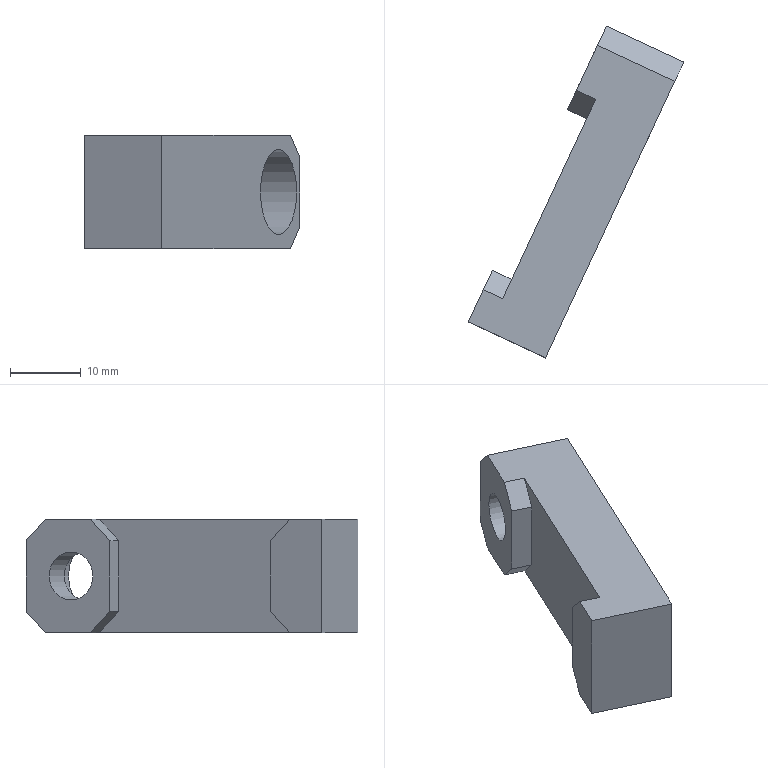Part | STEP file | gslz 2016.10.28-13_id454_x_t | 1 solid | 19 faces | box 30.316 x 46.762 x 16 mm | volume 6497 mm3 | plane 17 | cylinder 2 | commonest cylinder face diameters 6.8 x1 12 x1
STEP:
#1=CARTESIAN_POINT('',(0.,0.,0.));
#2=DIRECTION('',(0.,0.,1.));
#3=DIRECTION('',(1.,0.,0.));
#4=AXIS2_PLACEMENT_3D('',#1,#2,#3);
#5=CARTESIAN_POINT('',(887.546,-276.584,-28.));
#6=VERTEX_POINT('',#5);
#7=CARTESIAN_POINT('',(900.647,-248.489,-28.));
#8=VERTEX_POINT('',#7);
#9=CARTESIAN_POINT('',(891.35,-268.428,-28.));
#10=DIRECTION('',(0.4226,0.9063,0.));
#11=VECTOR('',#10,1.);
#12=LINE('',#9,#11);
#13=CARTESIAN_POINT('',(891.35,-268.428,-57.5));
#14=DIRECTION('',(0.9063,-0.4226,0.));
#15=DIRECTION('',(0.4226,0.9063,0.));
#16=AXIS2_PLACEMENT_3D('',#13,#14,#15);
#17=PLANE('',#16);
#18=CARTESIAN_POINT('',(0.,29.5));
#19=DIRECTION('',(1.,0.));
#20=VECTOR('',#19,1.);
#21=LINE('',#18,#20);
#22=(GEOMETRIC_REPRESENTATION_CONTEXT(2)PARAMETRIC_REPRESENTATION_CONTEXT()REPRESENTATION_CONTEXT('',''));
#23=DEFINITIONAL_REPRESENTATION('',(#21),#22);
#24=PCURVE('',#17,#23);
#25=CARTESIAN_POINT('',(900.413,-272.654,-28.));
#26=DIRECTION('',(0.,0.,-1.));
#27=DIRECTION('',(0.9397,-0.342,0.));
#28=AXIS2_PLACEMENT_3D('',#25,#26,#27);
#29=PLANE('',#28);
#30=CARTESIAN_POINT('',(-9.962,-0.8716));
#31=DIRECTION('',(0.08716,-0.9962));
#32=VECTOR('',#31,1.);
#33=LINE('',#30,#32);
#34=(GEOMETRIC_REPRESENTATION_CONTEXT(2)PARAMETRIC_REPRESENTATION_CONTEXT()REPRESENTATION_CONTEXT('',''));
#35=DEFINITIONAL_REPRESENTATION('',(#33),#34);
#36=PCURVE('',#29,#35);
#37=SURFACE_CURVE('',#12,(#24,#36),.PCURVE_S1.);
#38=EDGE_CURVE('',#6,#8,#37,.T.);
#39=ORIENTED_EDGE('',*,*,#38,.T.);
#40=CARTESIAN_POINT('',(899.379,-251.208,-31.));
#41=VERTEX_POINT('',#40);
#42=CARTESIAN_POINT('',(889.765,-271.826,-53.75));
#43=DIRECTION('',(0.2988,0.6409,0.7071));
#44=VECTOR('',#43,1.);
#45=LINE('',#42,#44);
#46=CARTESIAN_POINT('',(-3.75,3.75));
#47=DIRECTION('',(0.7071,0.7071));
#48=VECTOR('',#47,1.);
#49=LINE('',#46,#48);
#50=(GEOMETRIC_REPRESENTATION_CONTEXT(2)PARAMETRIC_REPRESENTATION_CONTEXT()REPRESENTATION_CONTEXT('',''));
#51=DEFINITIONAL_REPRESENTATION('',(#49),#50);
#52=PCURVE('',#17,#51);
#53=CARTESIAN_POINT('',(909.71,-252.715,-28.));
#54=DIRECTION('',(0.2988,0.6409,-0.7071));
#55=DIRECTION('',(-0.9063,0.4226,0.));
#56=AXIS2_PLACEMENT_3D('',#53,#54,#55);
#57=PLANE('',#56);
#58=CARTESIAN_POINT('',(10.,-36.416));
#59=DIRECTION('',(0.,1.));
#60=VECTOR('',#59,1.);
#61=LINE('',#58,#60);
#62=(GEOMETRIC_REPRESENTATION_CONTEXT(2)PARAMETRIC_REPRESENTATION_CONTEXT()REPRESENTATION_CONTEXT('',''));
#63=DEFINITIONAL_REPRESENTATION('',(#61),#62);
#64=PCURVE('',#57,#63);
#65=SURFACE_CURVE('',#45,(#52,#64),.PCURVE_S1.);
#66=EDGE_CURVE('',#41,#8,#65,.T.);
#67=ORIENTED_EDGE('',*,*,#66,.F.);
#68=CARTESIAN_POINT('',(899.379,-251.208,-41.));
#69=VERTEX_POINT('',#68);
#70=CARTESIAN_POINT('',(899.379,-251.208,-57.5));
#71=DIRECTION('',(0.,0.,1.));
#72=VECTOR('',#71,1.);
#73=LINE('',#70,#72);
#74=CARTESIAN_POINT('',(19.,0.));
#75=DIRECTION('',(0.,1.));
#76=VECTOR('',#75,1.);
#77=LINE('',#74,#76);
#78=(GEOMETRIC_REPRESENTATION_CONTEXT(2)PARAMETRIC_REPRESENTATION_CONTEXT()REPRESENTATION_CONTEXT('',''));
#79=DEFINITIONAL_REPRESENTATION('',(#77),#78);
#80=PCURVE('',#17,#79);
#81=CARTESIAN_POINT('',(907.536,-255.011,-36.));
#82=DIRECTION('',(0.4226,0.9063,0.));
#83=DIRECTION('',(0.9063,-0.4226,0.));
#84=AXIS2_PLACEMENT_3D('',#81,#82,#83);
#85=PLANE('',#84);
#86=CARTESIAN_POINT('',(-9.,21.5));
#87=DIRECTION('',(0.,-1.));
#88=VECTOR('',#87,1.);
#89=LINE('',#86,#88);
#90=(GEOMETRIC_REPRESENTATION_CONTEXT(2)PARAMETRIC_REPRESENTATION_CONTEXT()REPRESENTATION_CONTEXT('',''));
#91=DEFINITIONAL_REPRESENTATION('',(#89),#90);
#92=PCURVE('',#85,#91);
#93=SURFACE_CURVE('',#73,(#80,#92),.PCURVE_S1.);
#94=EDGE_CURVE('',#69,#41,#93,.T.);
#95=ORIENTED_EDGE('',*,*,#94,.F.);
#96=CARTESIAN_POINT('',(900.647,-248.489,-44.));
#97=VERTEX_POINT('',#96);
#98=CARTESIAN_POINT('',(898.851,-252.341,-39.75));
#99=DIRECTION('',(-0.2988,-0.6409,0.7071));
#100=VECTOR('',#99,1.);
#101=LINE('',#98,#100);
#102=CARTESIAN_POINT('',(17.75,17.75));
#103=DIRECTION('',(-0.7071,0.7071));
#104=VECTOR('',#103,1.);
#105=LINE('',#102,#104);
#106=(GEOMETRIC_REPRESENTATION_CONTEXT(2)PARAMETRIC_REPRESENTATION_CONTEXT()REPRESENTATION_CONTEXT('',''));
#107=DEFINITIONAL_REPRESENTATION('',(#105),#106);
#108=PCURVE('',#17,#107);
#109=CARTESIAN_POINT('',(907.536,-255.011,-41.));
#110=DIRECTION('',(-0.2988,-0.6409,-0.7071));
#111=DIRECTION('',(0.9063,-0.4226,0.));
#112=AXIS2_PLACEMENT_3D('',#109,#110,#111);
#113=PLANE('',#112);
#114=CARTESIAN_POINT('',(-9.,1.768));
#115=DIRECTION('',(0.,1.));
#116=VECTOR('',#115,1.);
#117=LINE('',#114,#116);
#118=(GEOMETRIC_REPRESENTATION_CONTEXT(2)PARAMETRIC_REPRESENTATION_CONTEXT()REPRESENTATION_CONTEXT('',''));
#119=DEFINITIONAL_REPRESENTATION('',(#117),#118);
#120=PCURVE('',#113,#119);
#121=SURFACE_CURVE('',#101,(#108,#120),.PCURVE_S1.);
#122=EDGE_CURVE('',#97,#69,#121,.T.);
#123=ORIENTED_EDGE('',*,*,#122,.F.);
#124=CARTESIAN_POINT('',(887.546,-276.584,-44.));
#125=VERTEX_POINT('',#124);
#126=CARTESIAN_POINT('',(891.35,-268.428,-44.));
#127=DIRECTION('',(0.4226,0.9063,0.));
#128=VECTOR('',#127,1.);
#129=LINE('',#126,#128);
#130=CARTESIAN_POINT('',(0.,13.5));
#131=DIRECTION('',(1.,0.));
#132=VECTOR('',#131,1.);
#133=LINE('',#130,#132);
#134=(GEOMETRIC_REPRESENTATION_CONTEXT(2)PARAMETRIC_REPRESENTATION_CONTEXT()REPRESENTATION_CONTEXT('',''));
#135=DEFINITIONAL_REPRESENTATION('',(#133),#134);
#136=PCURVE('',#17,#135);
#137=CARTESIAN_POINT('',(900.413,-272.654,-44.));
#138=DIRECTION('',(0.,0.,-1.));
#139=DIRECTION('',(0.9397,-0.342,0.));
#140=AXIS2_PLACEMENT_3D('',#137,#138,#139);
#141=PLANE('',#140);
#142=CARTESIAN_POINT('',(-9.962,-0.8716));
#143=DIRECTION('',(0.08716,-0.9962));
#144=VECTOR('',#143,1.);
#145=LINE('',#142,#144);
#146=(GEOMETRIC_REPRESENTATION_CONTEXT(2)PARAMETRIC_REPRESENTATION_CONTEXT()REPRESENTATION_CONTEXT('',''));
#147=DEFINITIONAL_REPRESENTATION('',(#145),#146);
#148=PCURVE('',#141,#147);
#149=SURFACE_CURVE('',#129,(#136,#148),.PCURVE_S1.);
#150=EDGE_CURVE('',#125,#97,#149,.T.);
#151=ORIENTED_EDGE('',*,*,#150,.F.);
#152=CARTESIAN_POINT('',(888.814,-273.865,-41.));
#153=VERTEX_POINT('',#152);
#154=CARTESIAN_POINT('',(886.595,-278.624,-46.25));
#155=DIRECTION('',(-0.2988,-0.6409,-0.7071));
#156=VECTOR('',#155,1.);
#157=LINE('',#154,#156);
#158=CARTESIAN_POINT('',(-11.25,11.25));
#159=DIRECTION('',(-0.7071,-0.7071));
#160=VECTOR('',#159,1.);
#161=LINE('',#158,#160);
#162=(GEOMETRIC_REPRESENTATION_CONTEXT(2)PARAMETRIC_REPRESENTATION_CONTEXT()REPRESENTATION_CONTEXT('',''));
#163=DEFINITIONAL_REPRESENTATION('',(#161),#162);
#164=PCURVE('',#17,#163);
#165=CARTESIAN_POINT('',(896.609,-280.811,-44.));
#166=DIRECTION('',(0.2988,0.6409,-0.7071));
#167=DIRECTION('',(0.9063,-0.4226,0.));
#168=AXIS2_PLACEMENT_3D('',#165,#166,#167);
#169=PLANE('',#168);
#170=CARTESIAN_POINT('',(-10.,3.182));
#171=DIRECTION('',(0.,1.));
#172=VECTOR('',#171,1.);
#173=LINE('',#170,#172);
#174=(GEOMETRIC_REPRESENTATION_CONTEXT(2)PARAMETRIC_REPRESENTATION_CONTEXT()REPRESENTATION_CONTEXT('',''));
#175=DEFINITIONAL_REPRESENTATION('',(#173),#174);
#176=PCURVE('',#169,#175);
#177=SURFACE_CURVE('',#157,(#164,#176),.PCURVE_S1.);
#178=EDGE_CURVE('',#153,#125,#177,.T.);
#179=ORIENTED_EDGE('',*,*,#178,.F.);
#180=CARTESIAN_POINT('',(888.814,-273.865,-31.));
#181=VERTEX_POINT('',#180);
#182=CARTESIAN_POINT('',(888.814,-273.865,-57.5));
#183=DIRECTION('',(0.,0.,1.));
#184=VECTOR('',#183,1.);
#185=LINE('',#182,#184);
#186=CARTESIAN_POINT('',(-6.,0.));
#187=DIRECTION('',(0.,1.));
#188=VECTOR('',#187,1.);
#189=LINE('',#186,#188);
#190=(GEOMETRIC_REPRESENTATION_CONTEXT(2)PARAMETRIC_REPRESENTATION_CONTEXT()REPRESENTATION_CONTEXT('',''));
#191=DEFINITIONAL_REPRESENTATION('',(#189),#190);
#192=PCURVE('',#17,#191);
#193=CARTESIAN_POINT('',(896.971,-277.669,-36.));
#194=DIRECTION('',(-0.4226,-0.9063,0.));
#195=DIRECTION('',(0.9063,-0.4226,0.));
#196=AXIS2_PLACEMENT_3D('',#193,#194,#195);
#197=PLANE('',#196);
#198=CARTESIAN_POINT('',(-9.,-21.5));
#199=DIRECTION('',(0.,1.));
#200=VECTOR('',#199,1.);
#201=LINE('',#198,#200);
#202=(GEOMETRIC_REPRESENTATION_CONTEXT(2)PARAMETRIC_REPRESENTATION_CONTEXT()REPRESENTATION_CONTEXT('',''));
#203=DEFINITIONAL_REPRESENTATION('',(#201),#202);
#204=PCURVE('',#197,#203);
#205=SURFACE_CURVE('',#185,(#192,#204),.PCURVE_S1.);
#206=EDGE_CURVE('',#153,#181,#205,.T.);
#207=ORIENTED_EDGE('',*,*,#206,.T.);
#208=CARTESIAN_POINT('',(895.681,-259.138,-47.25));
#209=DIRECTION('',(0.2988,0.6409,-0.7071));
#210=VECTOR('',#209,1.);
#211=LINE('',#208,#210);
#212=CARTESIAN_POINT('',(10.25,10.25));
#213=DIRECTION('',(0.7071,-0.7071));
#214=VECTOR('',#213,1.);
#215=LINE('',#212,#214);
#216=(GEOMETRIC_REPRESENTATION_CONTEXT(2)PARAMETRIC_REPRESENTATION_CONTEXT()REPRESENTATION_CONTEXT('',''));
#217=DEFINITIONAL_REPRESENTATION('',(#215),#216);
#218=PCURVE('',#17,#217);
#219=CARTESIAN_POINT('',(896.971,-277.669,-31.));
#220=DIRECTION('',(-0.2988,-0.6409,-0.7071));
#221=DIRECTION('',(-0.9063,0.4226,0.));
#222=AXIS2_PLACEMENT_3D('',#219,#220,#221);
#223=PLANE('',#222);
#224=CARTESIAN_POINT('',(9.,22.981));
#225=DIRECTION('',(0.,1.));
#226=VECTOR('',#225,1.);
#227=LINE('',#224,#226);
#228=(GEOMETRIC_REPRESENTATION_CONTEXT(2)PARAMETRIC_REPRESENTATION_CONTEXT()REPRESENTATION_CONTEXT('',''));
#229=DEFINITIONAL_REPRESENTATION('',(#227),#228);
#230=PCURVE('',#223,#229);
#231=SURFACE_CURVE('',#211,(#218,#230),.PCURVE_S1.);
#232=EDGE_CURVE('',#6,#181,#231,.T.);
#233=ORIENTED_EDGE('',*,*,#232,.F.);
#234=EDGE_LOOP('',(#39,#67,#95,#123,#151,#179,#207,#233));
#235=FACE_BOUND('',#234,.T.);
#236=ADVANCED_FACE('',(#235),#17,.F.);
#237=CARTESIAN_POINT('',(905.165,-243.534,-36.));
#238=VERTEX_POINT('',#237);
#239=CARTESIAN_POINT('',(903.728,-246.615,-36.));
#240=DIRECTION('',(0.9063,-0.4226,0.));
#241=DIRECTION('',(0.4226,0.9063,0.));
#242=AXIS2_PLACEMENT_3D('',#239,#240,#241);
#243=CIRCLE('',#242,3.4);
#244=CARTESIAN_POINT('',(817.628,-206.466,-36.));
#245=DIRECTION('',(-0.9063,0.4226,0.));
#246=DIRECTION('',(-0.4226,-0.9063,0.));
#247=AXIS2_PLACEMENT_3D('',#244,#245,#246);
#248=CYLINDRICAL_SURFACE('',#247,3.4);
#249=CARTESIAN_POINT('',(9.425,-95.));
#250=DIRECTION('',(-1.,0.));
#251=VECTOR('',#250,1.);
#252=LINE('',#249,#251);
#253=(GEOMETRIC_REPRESENTATION_CONTEXT(2)PARAMETRIC_REPRESENTATION_CONTEXT()REPRESENTATION_CONTEXT('',''));
#254=DEFINITIONAL_REPRESENTATION('',(#252),#253);
#255=PCURVE('',#248,#254);
#256=CARTESIAN_POINT('',(906.686,-240.271,-36.));
#257=DIRECTION('',(-0.9063,0.4226,0.));
#258=DIRECTION('',(-0.4226,-0.9063,0.));
#259=AXIS2_PLACEMENT_3D('',#256,#257,#258);
#260=PLANE('',#259);
#261=CARTESIAN_POINT('',(3.6,-0.000000001));
#262=CARTESIAN_POINT('',(3.6,5.889));
#263=CARTESIAN_POINT('',(8.7,2.944));
#264=CARTESIAN_POINT('',(13.8,0.000000001));
#265=CARTESIAN_POINT('',(8.7,-2.944));
#266=CARTESIAN_POINT('',(3.6,-5.889));
#267=CARTESIAN_POINT('',(3.6,-0.000000001));
#268=(BOUNDED_CURVE()B_SPLINE_CURVE(2,(#261,#262,#263,#264,#265,#266,#267),.UNSPECIFIED.,.T.,.F.)B_SPLINE_CURVE_WITH_KNOTS((1,2,2,2,2,1),(-2.094,0.,2.094,4.189,6.283,8.378),.UNSPECIFIED.)CURVE()GEOMETRIC_REPRESENTATION_ITEM()RATIONAL_B_SPLINE_CURVE((1.,0.5,1.,0.5,1.,0.5,1.))REPRESENTATION_ITEM(''));
#269=(GEOMETRIC_REPRESENTATION_CONTEXT(2)PARAMETRIC_REPRESENTATION_CONTEXT()REPRESENTATION_CONTEXT('',''));
#270=DEFINITIONAL_REPRESENTATION('',(#268),#269);
#271=PCURVE('',#260,#270);
#272=SURFACE_CURVE('',#243,(#255,#271),.PCURVE_S1.);
#273=EDGE_CURVE('',#238,#238,#272,.T.);
#274=ORIENTED_EDGE('',*,*,#273,.F.);
#275=CARTESIAN_POINT('',(900.633,-241.421,-36.));
#276=VERTEX_POINT('',#275);
#277=CARTESIAN_POINT('',(905.165,-243.534,-36.));
#278=CARTESIAN_POINT('',(900.633,-241.421,-36.));
#279=B_SPLINE_CURVE_WITH_KNOTS('',1,(#277,#278),.UNSPECIFIED.,.F.,.F.,(2,2),(-95.,-90.),.PIECEWISE_BEZIER_KNOTS.);
#280=CARTESIAN_POINT('',(9.425,0.));
#281=DIRECTION('',(0.,1.));
#282=VECTOR('',#281,1.);
#283=LINE('',#280,#282);
#284=(GEOMETRIC_REPRESENTATION_CONTEXT(2)PARAMETRIC_REPRESENTATION_CONTEXT()REPRESENTATION_CONTEXT('',''));
#285=DEFINITIONAL_REPRESENTATION('',(#283),#284);
#286=PCURVE('',#248,#285);
#287=CARTESIAN_POINT('',(3.142,0.));
#288=DIRECTION('',(0.,1.));
#289=VECTOR('',#288,1.);
#290=LINE('',#287,#289);
#291=(GEOMETRIC_REPRESENTATION_CONTEXT(2)PARAMETRIC_REPRESENTATION_CONTEXT()REPRESENTATION_CONTEXT('',''));
#292=DEFINITIONAL_REPRESENTATION('',(#290),#291);
#293=PCURVE('',#248,#292);
#294=SEAM_CURVE('',#279,(#286,#293),.PCURVE_S1.);
#295=EDGE_CURVE('',#238,#276,#294,.T.);
#296=ORIENTED_EDGE('',*,*,#295,.T.);
#297=CARTESIAN_POINT('',(899.196,-244.502,-36.));
#298=DIRECTION('',(-0.9063,0.4226,0.));
#299=DIRECTION('',(0.4226,0.9063,0.));
#300=AXIS2_PLACEMENT_3D('',#297,#298,#299);
#301=CIRCLE('',#300,3.4);
#302=CARTESIAN_POINT('',(3.142,-90.));
#303=DIRECTION('',(1.,0.));
#304=VECTOR('',#303,1.);
#305=LINE('',#302,#304);
#306=(GEOMETRIC_REPRESENTATION_CONTEXT(2)PARAMETRIC_REPRESENTATION_CONTEXT()REPRESENTATION_CONTEXT('',''));
#307=DEFINITIONAL_REPRESENTATION('',(#305),#306);
#308=PCURVE('',#248,#307);
#309=CARTESIAN_POINT('',(903.,-236.345,-57.5));
#310=DIRECTION('',(0.9063,-0.4226,0.));
#311=DIRECTION('',(-0.4226,-0.9063,0.));
#312=AXIS2_PLACEMENT_3D('',#309,#310,#311);
#313=PLANE('',#312);
#314=CARTESIAN_POINT('',(5.6,-21.5));
#315=CARTESIAN_POINT('',(5.6,-15.611));
#316=CARTESIAN_POINT('',(10.7,-18.556));
#317=CARTESIAN_POINT('',(15.8,-21.5));
#318=CARTESIAN_POINT('',(10.7,-24.444));
#319=CARTESIAN_POINT('',(5.6,-27.389));
#320=CARTESIAN_POINT('',(5.6,-21.5));
#321=(BOUNDED_CURVE()B_SPLINE_CURVE(2,(#314,#315,#316,#317,#318,#319,#320),.UNSPECIFIED.,.T.,.F.)B_SPLINE_CURVE_WITH_KNOTS((1,2,2,2,2,1),(-2.094,0.,2.094,4.189,6.283,8.378),.UNSPECIFIED.)CURVE()GEOMETRIC_REPRESENTATION_ITEM()RATIONAL_B_SPLINE_CURVE((1.,0.5,1.,0.5,1.,0.5,1.))REPRESENTATION_ITEM(''));
#322=(GEOMETRIC_REPRESENTATION_CONTEXT(2)PARAMETRIC_REPRESENTATION_CONTEXT()REPRESENTATION_CONTEXT('',''));
#323=DEFINITIONAL_REPRESENTATION('',(#321),#322);
#324=PCURVE('',#313,#323);
#325=SURFACE_CURVE('',#301,(#308,#324),.PCURVE_S1.);
#326=EDGE_CURVE('',#276,#276,#325,.T.);
#327=ORIENTED_EDGE('',*,*,#326,.F.);
#328=ORIENTED_EDGE('',*,*,#295,.F.);
#329=EDGE_LOOP('',(#274,#296,#327,#328));
#330=FACE_BOUND('',#329,.F.);
#331=ADVANCED_FACE('',(#330),#248,.F.);
#332=CARTESIAN_POINT('',(882.714,-279.848,-28.));
#333=VERTEX_POINT('',#332);
#334=CARTESIAN_POINT('',(884.827,-275.316,-28.));
#335=VERTEX_POINT('',#334);
#336=CARTESIAN_POINT('',(883.137,-278.942,-28.));
#337=DIRECTION('',(0.4226,0.9063,0.));
#338=VECTOR('',#337,1.);
#339=LINE('',#336,#338);
#340=CARTESIAN_POINT('',(-14.084,11.818));
#341=DIRECTION('',(0.08716,-0.9962));
#342=VECTOR('',#341,1.);
#343=LINE('',#340,#342);
#344=(GEOMETRIC_REPRESENTATION_CONTEXT(2)PARAMETRIC_REPRESENTATION_CONTEXT()REPRESENTATION_CONTEXT('',''));
#345=DEFINITIONAL_REPRESENTATION('',(#343),#344);
#346=PCURVE('',#29,#345);
#347=CARTESIAN_POINT('',(885.25,-274.41,-57.5));
#348=DIRECTION('',(0.9063,-0.4226,0.));
#349=DIRECTION('',(0.4226,0.9063,0.));
#350=AXIS2_PLACEMENT_3D('',#347,#348,#349);
#351=PLANE('',#350);
#352=CARTESIAN_POINT('',(-5.,29.5));
#353=DIRECTION('',(1.,0.));
#354=VECTOR('',#353,1.);
#355=LINE('',#352,#354);
#356=(GEOMETRIC_REPRESENTATION_CONTEXT(2)PARAMETRIC_REPRESENTATION_CONTEXT()REPRESENTATION_CONTEXT('',''));
#357=DEFINITIONAL_REPRESENTATION('',(#355),#356);
#358=PCURVE('',#351,#357);
#359=SURFACE_CURVE('',#339,(#346,#358),.PCURVE_S1.);
#360=EDGE_CURVE('',#333,#335,#359,.T.);
#361=ORIENTED_EDGE('',*,*,#360,.F.);
#362=CARTESIAN_POINT('',(893.59,-284.919,-28.));
#363=VERTEX_POINT('',#362);
#364=CARTESIAN_POINT('',(894.496,-285.342,-28.));
#365=DIRECTION('',(0.9063,-0.4226,0.));
#366=VECTOR('',#365,1.);
#367=LINE('',#364,#366);
#368=CARTESIAN_POINT('',(-1.22,13.947));
#369=DIRECTION('',(0.9962,0.08716));
#370=VECTOR('',#369,1.);
#371=LINE('',#368,#370);
#372=(GEOMETRIC_REPRESENTATION_CONTEXT(2)PARAMETRIC_REPRESENTATION_CONTEXT()REPRESENTATION_CONTEXT('',''));
#373=DEFINITIONAL_REPRESENTATION('',(#371),#372);
#374=PCURVE('',#29,#373);
#375=CARTESIAN_POINT('',(894.496,-285.342,-57.5));
#376=DIRECTION('',(-0.4226,-0.9063,0.));
#377=DIRECTION('',(0.9063,-0.4226,0.));
#378=AXIS2_PLACEMENT_3D('',#375,#376,#377);
#379=PLANE('',#378);
#380=CARTESIAN_POINT('',(0.,29.5));
#381=DIRECTION('',(1.,0.));
#382=VECTOR('',#381,1.);
#383=LINE('',#380,#382);
#384=(GEOMETRIC_REPRESENTATION_CONTEXT(2)PARAMETRIC_REPRESENTATION_CONTEXT()REPRESENTATION_CONTEXT('',''));
#385=DEFINITIONAL_REPRESENTATION('',(#383),#384);
#386=PCURVE('',#379,#385);
#387=SURFACE_CURVE('',#367,(#374,#386),.PCURVE_S1.);
#388=EDGE_CURVE('',#333,#363,#387,.T.);
#389=ORIENTED_EDGE('',*,*,#388,.T.);
#390=CARTESIAN_POINT('',(911.762,-245.948,-28.));
#391=VERTEX_POINT('',#390);
#392=CARTESIAN_POINT('',(899.506,-272.231,-28.));
#393=DIRECTION('',(0.4226,0.9063,0.));
#394=VECTOR('',#393,1.);
#395=LINE('',#392,#394);
#396=CARTESIAN_POINT('',(-0.9962,-0.08716));
#397=DIRECTION('',(0.08716,-0.9962));
#398=VECTOR('',#397,1.);
#399=LINE('',#396,#398);
#400=(GEOMETRIC_REPRESENTATION_CONTEXT(2)PARAMETRIC_REPRESENTATION_CONTEXT()REPRESENTATION_CONTEXT('',''));
#401=DEFINITIONAL_REPRESENTATION('',(#399),#400);
#402=PCURVE('',#29,#401);
#403=CARTESIAN_POINT('',(899.506,-272.231,-57.5));
#404=DIRECTION('',(0.9063,-0.4226,0.));
#405=DIRECTION('',(0.4226,0.9063,0.));
#406=AXIS2_PLACEMENT_3D('',#403,#404,#405);
#407=PLANE('',#406);
#408=CARTESIAN_POINT('',(0.,29.5));
#409=DIRECTION('',(1.,0.));
#410=VECTOR('',#409,1.);
#411=LINE('',#408,#410);
#412=(GEOMETRIC_REPRESENTATION_CONTEXT(2)PARAMETRIC_REPRESENTATION_CONTEXT()REPRESENTATION_CONTEXT('',''));
#413=DEFINITIONAL_REPRESENTATION('',(#411),#412);
#414=PCURVE('',#407,#413);
#415=SURFACE_CURVE('',#395,(#402,#414),.PCURVE_S1.);
#416=EDGE_CURVE('',#363,#391,#415,.T.);
#417=ORIENTED_EDGE('',*,*,#416,.T.);
#418=CARTESIAN_POINT('',(900.887,-240.877,-28.));
#419=VERTEX_POINT('',#418);
#420=CARTESIAN_POINT('',(900.887,-240.877,-28.));
#421=DIRECTION('',(-0.9063,0.4226,0.));
#422=VECTOR('',#421,1.);
#423=LINE('',#420,#422);
#424=CARTESIAN_POINT('',(-10.423,-30.023));
#425=DIRECTION('',(-0.9962,-0.08716));
#426=VECTOR('',#425,1.);
#427=LINE('',#424,#426);
#428=(GEOMETRIC_REPRESENTATION_CONTEXT(2)PARAMETRIC_REPRESENTATION_CONTEXT()REPRESENTATION_CONTEXT('',''));
#429=DEFINITIONAL_REPRESENTATION('',(#427),#428);
#430=PCURVE('',#29,#429);
#431=CARTESIAN_POINT('',(913.936,-243.652,-31.));
#432=DIRECTION('',(0.2988,0.6409,0.7071));
#433=DIRECTION('',(-0.9063,0.4226,0.));
#434=AXIS2_PLACEMENT_3D('',#431,#432,#433);
#435=PLANE('',#434);
#436=CARTESIAN_POINT('',(13.,4.243));
#437=DIRECTION('',(1.,0.));
#438=VECTOR('',#437,1.);
#439=LINE('',#436,#438);
#440=(GEOMETRIC_REPRESENTATION_CONTEXT(2)PARAMETRIC_REPRESENTATION_CONTEXT()REPRESENTATION_CONTEXT('',''));
#441=DEFINITIONAL_REPRESENTATION('',(#439),#440);
#442=PCURVE('',#435,#441);
#443=SURFACE_CURVE('',#423,(#430,#442),.PCURVE_S1.);
#444=EDGE_CURVE('',#391,#419,#443,.T.);
#445=ORIENTED_EDGE('',*,*,#444,.T.);
#446=CARTESIAN_POINT('',(897.928,-247.221,-28.));
#447=VERTEX_POINT('',#446);
#448=CARTESIAN_POINT('',(905.113,-231.814,-28.));
#449=DIRECTION('',(-0.4226,-0.9063,0.));
#450=VECTOR('',#449,1.);
#451=LINE('',#448,#450);
#452=CARTESIAN_POINT('',(-9.551,-39.985));
#453=DIRECTION('',(-0.08716,0.9962));
#454=VECTOR('',#453,1.);
#455=LINE('',#452,#454);
#456=(GEOMETRIC_REPRESENTATION_CONTEXT(2)PARAMETRIC_REPRESENTATION_CONTEXT()REPRESENTATION_CONTEXT('',''));
#457=DEFINITIONAL_REPRESENTATION('',(#455),#456);
#458=PCURVE('',#29,#457);
#459=CARTESIAN_POINT('',(-5.,-29.5));
#460=DIRECTION('',(1.,0.));
#461=VECTOR('',#460,1.);
#462=LINE('',#459,#461);
#463=(GEOMETRIC_REPRESENTATION_CONTEXT(2)PARAMETRIC_REPRESENTATION_CONTEXT()REPRESENTATION_CONTEXT('',''));
#464=DEFINITIONAL_REPRESENTATION('',(#462),#463);
#465=PCURVE('',#313,#464);
#466=SURFACE_CURVE('',#451,(#458,#465),.PCURVE_S1.);
#467=EDGE_CURVE('',#419,#447,#466,.T.);
#468=ORIENTED_EDGE('',*,*,#467,.T.);
#469=CARTESIAN_POINT('',(909.71,-252.715,-28.));
#470=DIRECTION('',(-0.9063,0.4226,0.));
#471=VECTOR('',#470,1.);
#472=LINE('',#469,#471);
#473=CARTESIAN_POINT('',(1.917,-21.916));
#474=DIRECTION('',(-0.9962,-0.08716));
#475=VECTOR('',#474,1.);
#476=LINE('',#473,#475);
#477=(GEOMETRIC_REPRESENTATION_CONTEXT(2)PARAMETRIC_REPRESENTATION_CONTEXT()REPRESENTATION_CONTEXT('',''));
#478=DEFINITIONAL_REPRESENTATION('',(#476),#477);
#479=PCURVE('',#29,#478);
#480=CARTESIAN_POINT('',(0.,0.));
#481=DIRECTION('',(1.,0.));
#482=VECTOR('',#481,1.);
#483=LINE('',#480,#482);
#484=(GEOMETRIC_REPRESENTATION_CONTEXT(2)PARAMETRIC_REPRESENTATION_CONTEXT()REPRESENTATION_CONTEXT('',''));
#485=DEFINITIONAL_REPRESENTATION('',(#483),#484);
#486=PCURVE('',#57,#485);
#487=SURFACE_CURVE('',#472,(#479,#486),.PCURVE_S1.);
#488=EDGE_CURVE('',#8,#447,#487,.T.);
#489=ORIENTED_EDGE('',*,*,#488,.F.);
#490=ORIENTED_EDGE('',*,*,#38,.F.);
#491=CARTESIAN_POINT('',(896.609,-280.811,-28.));
#492=DIRECTION('',(0.9063,-0.4226,0.));
#493=VECTOR('',#492,1.);
#494=LINE('',#491,#493);
#495=CARTESIAN_POINT('',(-0.7844,8.966));
#496=DIRECTION('',(0.9962,0.08716));
#497=VECTOR('',#496,1.);
#498=LINE('',#495,#497);
#499=(GEOMETRIC_REPRESENTATION_CONTEXT(2)PARAMETRIC_REPRESENTATION_CONTEXT()REPRESENTATION_CONTEXT('',''));
#500=DEFINITIONAL_REPRESENTATION('',(#498),#499);
#501=PCURVE('',#29,#500);
#502=CARTESIAN_POINT('',(-1.,-4.243));
#503=DIRECTION('',(-1.,0.));
#504=VECTOR('',#503,1.);
#505=LINE('',#502,#504);
#506=(GEOMETRIC_REPRESENTATION_CONTEXT(2)PARAMETRIC_REPRESENTATION_CONTEXT()REPRESENTATION_CONTEXT('',''));
#507=DEFINITIONAL_REPRESENTATION('',(#505),#506);
#508=PCURVE('',#223,#507);
#509=SURFACE_CURVE('',#494,(#501,#508),.PCURVE_S1.);
#510=EDGE_CURVE('',#335,#6,#509,.T.);
#511=ORIENTED_EDGE('',*,*,#510,.F.);
#512=EDGE_LOOP('',(#361,#389,#417,#445,#468,#489,#490,#511));
#513=FACE_BOUND('',#512,.T.);
#514=ADVANCED_FACE('',(#513),#29,.F.);
#515=CARTESIAN_POINT('',(882.714,-279.848,-44.));
#516=VERTEX_POINT('',#515);
#517=CARTESIAN_POINT('',(882.714,-279.848,-57.5));
#518=DIRECTION('',(0.,0.,-1.));
#519=VECTOR('',#518,1.);
#520=LINE('',#517,#519);
#521=CARTESIAN_POINT('',(-13.,0.));
#522=DIRECTION('',(0.,-1.));
#523=VECTOR('',#522,1.);
#524=LINE('',#521,#523);
#525=(GEOMETRIC_REPRESENTATION_CONTEXT(2)PARAMETRIC_REPRESENTATION_CONTEXT()REPRESENTATION_CONTEXT('',''));
#526=DEFINITIONAL_REPRESENTATION('',(#524),#525);
#527=PCURVE('',#379,#526);
#528=CARTESIAN_POINT('',(-6.,0.));
#529=DIRECTION('',(0.,-1.));
#530=VECTOR('',#529,1.);
#531=LINE('',#528,#530);
#532=(GEOMETRIC_REPRESENTATION_CONTEXT(2)PARAMETRIC_REPRESENTATION_CONTEXT()REPRESENTATION_CONTEXT('',''));
#533=DEFINITIONAL_REPRESENTATION('',(#531),#532);
#534=PCURVE('',#351,#533);
#535=SURFACE_CURVE('',#520,(#527,#534),.PCURVE_S1.);
#536=EDGE_CURVE('',#333,#516,#535,.T.);
#537=ORIENTED_EDGE('',*,*,#536,.T.);
#538=CARTESIAN_POINT('',(893.59,-284.919,-44.));
#539=VERTEX_POINT('',#538);
#540=CARTESIAN_POINT('',(894.496,-285.342,-44.));
#541=DIRECTION('',(0.9063,-0.4226,0.));
#542=VECTOR('',#541,1.);
#543=LINE('',#540,#542);
#544=CARTESIAN_POINT('',(0.,13.5));
#545=DIRECTION('',(1.,0.));
#546=VECTOR('',#545,1.);
#547=LINE('',#544,#546);
#548=(GEOMETRIC_REPRESENTATION_CONTEXT(2)PARAMETRIC_REPRESENTATION_CONTEXT()REPRESENTATION_CONTEXT('',''));
#549=DEFINITIONAL_REPRESENTATION('',(#547),#548);
#550=PCURVE('',#379,#549);
#551=CARTESIAN_POINT('',(-1.22,13.947));
#552=DIRECTION('',(0.9962,0.08716));
#553=VECTOR('',#552,1.);
#554=LINE('',#551,#553);
#555=(GEOMETRIC_REPRESENTATION_CONTEXT(2)PARAMETRIC_REPRESENTATION_CONTEXT()REPRESENTATION_CONTEXT('',''));
#556=DEFINITIONAL_REPRESENTATION('',(#554),#555);
#557=PCURVE('',#141,#556);
#558=SURFACE_CURVE('',#543,(#550,#557),.PCURVE_S1.);
#559=EDGE_CURVE('',#516,#539,#558,.T.);
#560=ORIENTED_EDGE('',*,*,#559,.T.);
#561=CARTESIAN_POINT('',(893.59,-284.919,-57.5));
#562=DIRECTION('',(0.,0.,1.));
#563=VECTOR('',#562,1.);
#564=LINE('',#561,#563);
#565=CARTESIAN_POINT('',(-1.,0.));
#566=DIRECTION('',(0.,1.));
#567=VECTOR('',#566,1.);
#568=LINE('',#565,#567);
#569=(GEOMETRIC_REPRESENTATION_CONTEXT(2)PARAMETRIC_REPRESENTATION_CONTEXT()REPRESENTATION_CONTEXT('',''));
#570=DEFINITIONAL_REPRESENTATION('',(#568),#569);
#571=PCURVE('',#379,#570);
#572=CARTESIAN_POINT('',(-14.,0.));
#573=DIRECTION('',(0.,1.));
#574=VECTOR('',#573,1.);
#575=LINE('',#572,#574);
#576=(GEOMETRIC_REPRESENTATION_CONTEXT(2)PARAMETRIC_REPRESENTATION_CONTEXT()REPRESENTATION_CONTEXT('',''));
#577=DEFINITIONAL_REPRESENTATION('',(#575),#576);
#578=PCURVE('',#407,#577);
#579=SURFACE_CURVE('',#564,(#571,#578),.PCURVE_S1.);
#580=EDGE_CURVE('',#539,#363,#579,.T.);
#581=ORIENTED_EDGE('',*,*,#580,.T.);
#582=ORIENTED_EDGE('',*,*,#388,.F.);
#583=EDGE_LOOP('',(#537,#560,#581,#582));
#584=FACE_BOUND('',#583,.T.);
#585=ADVANCED_FACE('',(#584),#379,.T.);
#586=ORIENTED_EDGE('',*,*,#150,.T.);
#587=CARTESIAN_POINT('',(897.928,-247.221,-44.));
#588=VERTEX_POINT('',#587);
#589=CARTESIAN_POINT('',(900.647,-248.489,-44.));
#590=DIRECTION('',(0.9063,-0.4226,0.));
#591=VECTOR('',#590,1.);
#592=LINE('',#589,#591);
#593=CARTESIAN_POINT('',(-8.045,-22.788));
#594=DIRECTION('',(0.9962,0.08716));
#595=VECTOR('',#594,1.);
#596=LINE('',#593,#595);
#597=(GEOMETRIC_REPRESENTATION_CONTEXT(2)PARAMETRIC_REPRESENTATION_CONTEXT()REPRESENTATION_CONTEXT('',''));
#598=DEFINITIONAL_REPRESENTATION('',(#596),#597);
#599=PCURVE('',#141,#598);
#600=CARTESIAN_POINT('',(-9.,-4.243));
#601=DIRECTION('',(1.,0.));
#602=VECTOR('',#601,1.);
#603=LINE('',#600,#602);
#604=(GEOMETRIC_REPRESENTATION_CONTEXT(2)PARAMETRIC_REPRESENTATION_CONTEXT()REPRESENTATION_CONTEXT('',''));
#605=DEFINITIONAL_REPRESENTATION('',(#603),#604);
#606=PCURVE('',#113,#605);
#607=SURFACE_CURVE('',#592,(#599,#606),.PCURVE_S1.);
#608=EDGE_CURVE('',#588,#97,#607,.T.);
#609=ORIENTED_EDGE('',*,*,#608,.F.);
#610=CARTESIAN_POINT('',(900.887,-240.877,-44.));
#611=VERTEX_POINT('',#610);
#612=CARTESIAN_POINT('',(905.113,-231.814,-44.));
#613=DIRECTION('',(-0.4226,-0.9063,0.));
#614=VECTOR('',#613,1.);
#615=LINE('',#612,#614);
#616=CARTESIAN_POINT('',(-9.551,-39.985));
#617=DIRECTION('',(-0.08716,0.9962));
#618=VECTOR('',#617,1.);
#619=LINE('',#616,#618);
#620=(GEOMETRIC_REPRESENTATION_CONTEXT(2)PARAMETRIC_REPRESENTATION_CONTEXT()REPRESENTATION_CONTEXT('',''));
#621=DEFINITIONAL_REPRESENTATION('',(#619),#620);
#622=PCURVE('',#141,#621);
#623=CARTESIAN_POINT('',(-5.,-13.5));
#624=DIRECTION('',(1.,0.));
#625=VECTOR('',#624,1.);
#626=LINE('',#623,#625);
#627=(GEOMETRIC_REPRESENTATION_CONTEXT(2)PARAMETRIC_REPRESENTATION_CONTEXT()REPRESENTATION_CONTEXT('',''));
#628=DEFINITIONAL_REPRESENTATION('',(#626),#627);
#629=PCURVE('',#313,#628);
#630=SURFACE_CURVE('',#615,(#622,#629),.PCURVE_S1.);
#631=EDGE_CURVE('',#611,#588,#630,.T.);
#632=ORIENTED_EDGE('',*,*,#631,.F.);
#633=CARTESIAN_POINT('',(911.762,-245.948,-44.));
#634=VERTEX_POINT('',#633);
#635=CARTESIAN_POINT('',(912.669,-246.371,-44.));
#636=DIRECTION('',(0.9063,-0.4226,0.));
#637=VECTOR('',#636,1.);
#638=LINE('',#635,#637);
#639=CARTESIAN_POINT('',(2.528,-28.89));
#640=DIRECTION('',(0.9962,0.08716));
#641=VECTOR('',#640,1.);
#642=LINE('',#639,#641);
#643=(GEOMETRIC_REPRESENTATION_CONTEXT(2)PARAMETRIC_REPRESENTATION_CONTEXT()REPRESENTATION_CONTEXT('',''));
#644=DEFINITIONAL_REPRESENTATION('',(#642),#643);
#645=PCURVE('',#141,#644);
#646=CARTESIAN_POINT('',(912.669,-246.371,-44.));
#647=DIRECTION('',(-0.2988,-0.6409,0.7071));
#648=DIRECTION('',(0.9063,-0.4226,0.));
#649=AXIS2_PLACEMENT_3D('',#646,#647,#648);
#650=PLANE('',#649);
#651=CARTESIAN_POINT('',(0.,0.));
#652=DIRECTION('',(1.,0.));
#653=VECTOR('',#652,1.);
#654=LINE('',#651,#653);
#655=(GEOMETRIC_REPRESENTATION_CONTEXT(2)PARAMETRIC_REPRESENTATION_CONTEXT()REPRESENTATION_CONTEXT('',''));
#656=DEFINITIONAL_REPRESENTATION('',(#654),#655);
#657=PCURVE('',#650,#656);
#658=SURFACE_CURVE('',#638,(#645,#657),.PCURVE_S1.);
#659=EDGE_CURVE('',#611,#634,#658,.T.);
#660=ORIENTED_EDGE('',*,*,#659,.T.);
#661=CARTESIAN_POINT('',(899.506,-272.231,-44.));
#662=DIRECTION('',(0.4226,0.9063,0.));
#663=VECTOR('',#662,1.);
#664=LINE('',#661,#663);
#665=CARTESIAN_POINT('',(-0.9962,-0.08716));
#666=DIRECTION('',(0.08716,-0.9962));
#667=VECTOR('',#666,1.);
#668=LINE('',#665,#667);
#669=(GEOMETRIC_REPRESENTATION_CONTEXT(2)PARAMETRIC_REPRESENTATION_CONTEXT()REPRESENTATION_CONTEXT('',''));
#670=DEFINITIONAL_REPRESENTATION('',(#668),#669);
#671=PCURVE('',#141,#670);
#672=CARTESIAN_POINT('',(0.,13.5));
#673=DIRECTION('',(1.,0.));
#674=VECTOR('',#673,1.);
#675=LINE('',#672,#674);
#676=(GEOMETRIC_REPRESENTATION_CONTEXT(2)PARAMETRIC_REPRESENTATION_CONTEXT()REPRESENTATION_CONTEXT('',''));
#677=DEFINITIONAL_REPRESENTATION('',(#675),#676);
#678=PCURVE('',#407,#677);
#679=SURFACE_CURVE('',#664,(#671,#678),.PCURVE_S1.);
#680=EDGE_CURVE('',#539,#634,#679,.T.);
#681=ORIENTED_EDGE('',*,*,#680,.F.);
#682=ORIENTED_EDGE('',*,*,#559,.F.);
#683=CARTESIAN_POINT('',(884.827,-275.316,-44.));
#684=VERTEX_POINT('',#683);
#685=CARTESIAN_POINT('',(883.137,-278.942,-44.));
#686=DIRECTION('',(0.4226,0.9063,0.));
#687=VECTOR('',#686,1.);
#688=LINE('',#685,#687);
#689=CARTESIAN_POINT('',(-14.084,11.818));
#690=DIRECTION('',(0.08716,-0.9962));
#691=VECTOR('',#690,1.);
#692=LINE('',#689,#691);
#693=(GEOMETRIC_REPRESENTATION_CONTEXT(2)PARAMETRIC_REPRESENTATION_CONTEXT()REPRESENTATION_CONTEXT('',''));
#694=DEFINITIONAL_REPRESENTATION('',(#692),#693);
#695=PCURVE('',#141,#694);
#696=CARTESIAN_POINT('',(-5.,13.5));
#697=DIRECTION('',(1.,0.));
#698=VECTOR('',#697,1.);
#699=LINE('',#696,#698);
#700=(GEOMETRIC_REPRESENTATION_CONTEXT(2)PARAMETRIC_REPRESENTATION_CONTEXT()REPRESENTATION_CONTEXT('',''));
#701=DEFINITIONAL_REPRESENTATION('',(#699),#700);
#702=PCURVE('',#351,#701);
#703=SURFACE_CURVE('',#688,(#695,#702),.PCURVE_S1.);
#704=EDGE_CURVE('',#516,#684,#703,.T.);
#705=ORIENTED_EDGE('',*,*,#704,.T.);
#706=CARTESIAN_POINT('',(884.827,-275.316,-44.));
#707=DIRECTION('',(-0.9063,0.4226,0.));
#708=VECTOR('',#707,1.);
#709=LINE('',#706,#708);
#710=CARTESIAN_POINT('',(-13.735,7.833));
#711=DIRECTION('',(-0.9962,-0.08716));
#712=VECTOR('',#711,1.);
#713=LINE('',#710,#712);
#714=(GEOMETRIC_REPRESENTATION_CONTEXT(2)PARAMETRIC_REPRESENTATION_CONTEXT()REPRESENTATION_CONTEXT('',''));
#715=DEFINITIONAL_REPRESENTATION('',(#713),#714);
#716=PCURVE('',#141,#715);
#717=CARTESIAN_POINT('',(-13.,0.));
#718=DIRECTION('',(-1.,0.));
#719=VECTOR('',#718,1.);
#720=LINE('',#717,#719);
#721=(GEOMETRIC_REPRESENTATION_CONTEXT(2)PARAMETRIC_REPRESENTATION_CONTEXT()REPRESENTATION_CONTEXT('',''));
#722=DEFINITIONAL_REPRESENTATION('',(#720),#721);
#723=PCURVE('',#169,#722);
#724=SURFACE_CURVE('',#709,(#716,#723),.PCURVE_S1.);
#725=EDGE_CURVE('',#125,#684,#724,.T.);
#726=ORIENTED_EDGE('',*,*,#725,.F.);
#727=EDGE_LOOP('',(#586,#609,#632,#660,#681,#682,#705,#726));
#728=FACE_BOUND('',#727,.T.);
#729=ADVANCED_FACE('',(#728),#141,.T.);
#730=ORIENTED_EDGE('',*,*,#580,.F.);
#731=ORIENTED_EDGE('',*,*,#680,.T.);
#732=CARTESIAN_POINT('',(913.03,-243.229,-41.));
#733=VERTEX_POINT('',#732);
#734=CARTESIAN_POINT('',(902.782,-265.207,-65.25));
#735=DIRECTION('',(0.2988,0.6409,0.7071));
#736=VECTOR('',#735,1.);
#737=LINE('',#734,#736);
#738=CARTESIAN_POINT('',(7.75,-7.75));
#739=DIRECTION('',(0.7071,0.7071));
#740=VECTOR('',#739,1.);
#741=LINE('',#738,#740);
#742=(GEOMETRIC_REPRESENTATION_CONTEXT(2)PARAMETRIC_REPRESENTATION_CONTEXT()REPRESENTATION_CONTEXT('',''));
#743=DEFINITIONAL_REPRESENTATION('',(#741),#742);
#744=PCURVE('',#407,#743);
#745=CARTESIAN_POINT('',(-1.,-30.052));
#746=DIRECTION('',(0.,1.));
#747=VECTOR('',#746,1.);
#748=LINE('',#745,#747);
#749=(GEOMETRIC_REPRESENTATION_CONTEXT(2)PARAMETRIC_REPRESENTATION_CONTEXT()REPRESENTATION_CONTEXT('',''));
#750=DEFINITIONAL_REPRESENTATION('',(#748),#749);
#751=PCURVE('',#650,#750);
#752=SURFACE_CURVE('',#737,(#744,#751),.PCURVE_S1.);
#753=EDGE_CURVE('',#634,#733,#752,.T.);
#754=ORIENTED_EDGE('',*,*,#753,.T.);
#755=CARTESIAN_POINT('',(913.03,-243.229,-31.));
#756=VERTEX_POINT('',#755);
#757=CARTESIAN_POINT('',(913.03,-243.229,-57.5));
#758=DIRECTION('',(0.,0.,-1.));
#759=VECTOR('',#758,1.);
#760=LINE('',#757,#759);
#761=CARTESIAN_POINT('',(32.,0.));
#762=DIRECTION('',(0.,-1.));
#763=VECTOR('',#762,1.);
#764=LINE('',#761,#763);
#765=(GEOMETRIC_REPRESENTATION_CONTEXT(2)PARAMETRIC_REPRESENTATION_CONTEXT()REPRESENTATION_CONTEXT('',''));
#766=DEFINITIONAL_REPRESENTATION('',(#764),#765);
#767=PCURVE('',#407,#766);
#768=CARTESIAN_POINT('',(913.936,-243.652,-57.5));
#769=DIRECTION('',(0.4226,0.9063,0.));
#770=DIRECTION('',(0.9063,-0.4226,0.));
#771=AXIS2_PLACEMENT_3D('',#768,#769,#770);
#772=PLANE('',#771);
#773=CARTESIAN_POINT('',(-1.,0.));
#774=DIRECTION('',(0.,1.));
#775=VECTOR('',#774,1.);
#776=LINE('',#773,#775);
#777=(GEOMETRIC_REPRESENTATION_CONTEXT(2)PARAMETRIC_REPRESENTATION_CONTEXT()REPRESENTATION_CONTEXT('',''));
#778=DEFINITIONAL_REPRESENTATION('',(#776),#777);
#779=PCURVE('',#772,#778);
#780=SURFACE_CURVE('',#760,(#767,#779),.PCURVE_S1.);
#781=EDGE_CURVE('',#756,#733,#780,.T.);
#782=ORIENTED_EDGE('',*,*,#781,.F.);
#783=CARTESIAN_POINT('',(911.868,-245.722,-28.25));
#784=DIRECTION('',(-0.2988,-0.6409,0.7071));
#785=VECTOR('',#784,1.);
#786=LINE('',#783,#785);
#787=CARTESIAN_POINT('',(29.25,29.25));
#788=DIRECTION('',(-0.7071,0.7071));
#789=VECTOR('',#788,1.);
#790=LINE('',#787,#789);
#791=(GEOMETRIC_REPRESENTATION_CONTEXT(2)PARAMETRIC_REPRESENTATION_CONTEXT()REPRESENTATION_CONTEXT('',''));
#792=DEFINITIONAL_REPRESENTATION('',(#790),#791);
#793=PCURVE('',#407,#792);
#794=CARTESIAN_POINT('',(1.,3.889));
#795=DIRECTION('',(0.,1.));
#796=VECTOR('',#795,1.);
#797=LINE('',#794,#796);
#798=(GEOMETRIC_REPRESENTATION_CONTEXT(2)PARAMETRIC_REPRESENTATION_CONTEXT()REPRESENTATION_CONTEXT('',''));
#799=DEFINITIONAL_REPRESENTATION('',(#797),#798);
#800=PCURVE('',#435,#799);
#801=SURFACE_CURVE('',#786,(#793,#800),.PCURVE_S1.);
#802=EDGE_CURVE('',#756,#391,#801,.T.);
#803=ORIENTED_EDGE('',*,*,#802,.T.);
#804=ORIENTED_EDGE('',*,*,#416,.F.);
#805=EDGE_LOOP('',(#730,#731,#754,#782,#803,#804));
#806=FACE_BOUND('',#805,.T.);
#807=CARTESIAN_POINT('',(907.536,-255.011,-36.));
#808=VERTEX_POINT('',#807);
#809=CARTESIAN_POINT('',(910.072,-249.573,-36.));
#810=DIRECTION('',(-0.9063,0.4226,0.));
#811=DIRECTION('',(-0.4226,-0.9063,0.));
#812=AXIS2_PLACEMENT_3D('',#809,#810,#811);
#813=CIRCLE('',#812,6.);
#814=CARTESIAN_POINT('',(19.,21.5));
#815=CARTESIAN_POINT('',(19.,31.892));
#816=CARTESIAN_POINT('',(28.,26.696));
#817=CARTESIAN_POINT('',(37.,21.5));
#818=CARTESIAN_POINT('',(28.,16.304));
#819=CARTESIAN_POINT('',(19.,11.108));
#820=CARTESIAN_POINT('',(19.,21.5));
#821=(BOUNDED_CURVE()B_SPLINE_CURVE(2,(#814,#815,#816,#817,#818,#819,#820),.UNSPECIFIED.,.T.,.F.)B_SPLINE_CURVE_WITH_KNOTS((1,2,2,2,2,1),(-2.094,0.,2.094,4.189,6.283,8.378),.UNSPECIFIED.)CURVE()GEOMETRIC_REPRESENTATION_ITEM()RATIONAL_B_SPLINE_CURVE((1.,0.5,1.,0.5,1.,0.5,1.))REPRESENTATION_ITEM(''));
#822=(GEOMETRIC_REPRESENTATION_CONTEXT(2)PARAMETRIC_REPRESENTATION_CONTEXT()REPRESENTATION_CONTEXT('',''));
#823=DEFINITIONAL_REPRESENTATION('',(#821),#822);
#824=PCURVE('',#407,#823);
#825=CARTESIAN_POINT('',(918.229,-253.377,-36.));
#826=DIRECTION('',(-0.9063,0.4226,0.));
#827=DIRECTION('',(-0.4226,-0.9063,0.));
#828=AXIS2_PLACEMENT_3D('',#825,#826,#827);
#829=CYLINDRICAL_SURFACE('',#828,6.);
#830=CARTESIAN_POINT('',(0.,9.));
#831=DIRECTION('',(1.,0.));
#832=VECTOR('',#831,1.);
#833=LINE('',#830,#832);
#834=(GEOMETRIC_REPRESENTATION_CONTEXT(2)PARAMETRIC_REPRESENTATION_CONTEXT()REPRESENTATION_CONTEXT('',''));
#835=DEFINITIONAL_REPRESENTATION('',(#833),#834);
#836=PCURVE('',#829,#835);
#837=SURFACE_CURVE('',#813,(#824,#836),.PCURVE_S1.);
#838=EDGE_CURVE('',#808,#808,#837,.T.);
#839=ORIENTED_EDGE('',*,*,#838,.T.);
#840=EDGE_LOOP('',(#839));
#841=FACE_BOUND('',#840,.T.);
#842=ADVANCED_FACE('',(#806,#841),#407,.T.);
#843=ORIENTED_EDGE('',*,*,#781,.T.);
#844=CARTESIAN_POINT('',(902.154,-238.158,-41.));
#845=VERTEX_POINT('',#844);
#846=CARTESIAN_POINT('',(913.936,-243.652,-41.));
#847=DIRECTION('',(-0.9063,0.4226,0.));
#848=VECTOR('',#847,1.);
#849=LINE('',#846,#848);
#850=CARTESIAN_POINT('',(0.,-16.5));
#851=DIRECTION('',(-1.,0.));
#852=VECTOR('',#851,1.);
#853=LINE('',#850,#852);
#854=(GEOMETRIC_REPRESENTATION_CONTEXT(2)PARAMETRIC_REPRESENTATION_CONTEXT()REPRESENTATION_CONTEXT('',''));
#855=DEFINITIONAL_REPRESENTATION('',(#853),#854);
#856=PCURVE('',#772,#855);
#857=CARTESIAN_POINT('',(0.,4.243));
#858=DIRECTION('',(-1.,0.));
#859=VECTOR('',#858,1.);
#860=LINE('',#857,#859);
#861=(GEOMETRIC_REPRESENTATION_CONTEXT(2)PARAMETRIC_REPRESENTATION_CONTEXT()REPRESENTATION_CONTEXT('',''));
#862=DEFINITIONAL_REPRESENTATION('',(#860),#861);
#863=PCURVE('',#650,#862);
#864=SURFACE_CURVE('',#849,(#856,#863),.PCURVE_S1.);
#865=EDGE_CURVE('',#733,#845,#864,.T.);
#866=ORIENTED_EDGE('',*,*,#865,.T.);
#867=CARTESIAN_POINT('',(902.154,-238.158,-31.));
#868=VERTEX_POINT('',#867);
#869=CARTESIAN_POINT('',(902.154,-238.158,-57.5));
#870=DIRECTION('',(0.,0.,-1.));
#871=VECTOR('',#870,1.);
#872=LINE('',#869,#871);
#873=CARTESIAN_POINT('',(-13.,0.));
#874=DIRECTION('',(0.,1.));
#875=VECTOR('',#874,1.);
#876=LINE('',#873,#875);
#877=(GEOMETRIC_REPRESENTATION_CONTEXT(2)PARAMETRIC_REPRESENTATION_CONTEXT()REPRESENTATION_CONTEXT('',''));
#878=DEFINITIONAL_REPRESENTATION('',(#876),#877);
#879=PCURVE('',#772,#878);
#880=CARTESIAN_POINT('',(2.,0.));
#881=DIRECTION('',(0.,1.));
#882=VECTOR('',#881,1.);
#883=LINE('',#880,#882);
#884=(GEOMETRIC_REPRESENTATION_CONTEXT(2)PARAMETRIC_REPRESENTATION_CONTEXT()REPRESENTATION_CONTEXT('',''));
#885=DEFINITIONAL_REPRESENTATION('',(#883),#884);
#886=PCURVE('',#313,#885);
#887=SURFACE_CURVE('',#872,(#879,#886),.PCURVE_S1.);
#888=EDGE_CURVE('',#868,#845,#887,.T.);
#889=ORIENTED_EDGE('',*,*,#888,.F.);
#890=CARTESIAN_POINT('',(915.749,-244.497,-31.));
#891=DIRECTION('',(0.9063,-0.4226,0.));
#892=VECTOR('',#891,1.);
#893=LINE('',#890,#892);
#894=CARTESIAN_POINT('',(2.,-26.5));
#895=DIRECTION('',(1.,0.));
#896=VECTOR('',#895,1.);
#897=LINE('',#894,#896);
#898=(GEOMETRIC_REPRESENTATION_CONTEXT(2)PARAMETRIC_REPRESENTATION_CONTEXT()REPRESENTATION_CONTEXT('',''));
#899=DEFINITIONAL_REPRESENTATION('',(#897),#898);
#900=PCURVE('',#772,#899);
#901=CARTESIAN_POINT('',(-2.,0.));
#902=DIRECTION('',(-1.,0.));
#903=VECTOR('',#902,1.);
#904=LINE('',#901,#903);
#905=(GEOMETRIC_REPRESENTATION_CONTEXT(2)PARAMETRIC_REPRESENTATION_CONTEXT()REPRESENTATION_CONTEXT('',''));
#906=DEFINITIONAL_REPRESENTATION('',(#904),#905);
#907=PCURVE('',#435,#906);
#908=SURFACE_CURVE('',#893,(#900,#907),.PCURVE_S1.);
#909=EDGE_CURVE('',#868,#756,#908,.T.);
#910=ORIENTED_EDGE('',*,*,#909,.T.);
#911=EDGE_LOOP('',(#843,#866,#889,#910));
#912=FACE_BOUND('',#911,.T.);
#913=ADVANCED_FACE('',(#912),#772,.T.);
#914=ORIENTED_EDGE('',*,*,#273,.F.);
#915=EDGE_LOOP('',(#914));
#916=FACE_BOUND('',#915,.T.);
#917=CARTESIAN_POINT('',(906.263,-241.177,-36.));
#918=VERTEX_POINT('',#917);
#919=CARTESIAN_POINT('',(901.192,-252.053,-36.));
#920=VERTEX_POINT('',#919);
#921=CARTESIAN_POINT('',(903.728,-246.615,-36.));
#922=DIRECTION('',(0.9063,-0.4226,0.));
#923=DIRECTION('',(0.4226,0.9063,0.));
#924=AXIS2_PLACEMENT_3D('',#921,#922,#923);
#925=CIRCLE('',#924,6.);
#926=CARTESIAN_POINT('',(1.,-0.000000001));
#927=CARTESIAN_POINT('',(1.,10.392));
#928=CARTESIAN_POINT('',(10.,5.196));
#929=CARTESIAN_POINT('',(19.,0.000000002));
#930=CARTESIAN_POINT('',(10.,-5.196));
#931=CARTESIAN_POINT('',(1.,-10.392));
#932=CARTESIAN_POINT('',(1.,-0.000000001));
#933=(BOUNDED_CURVE()B_SPLINE_CURVE(2,(#926,#927,#928,#929,#930,#931,#932),.UNSPECIFIED.,.T.,.F.)B_SPLINE_CURVE_WITH_KNOTS((1,2,2,2,2,1),(-2.094,0.,2.094,4.189,6.283,8.378),.UNSPECIFIED.)CURVE()GEOMETRIC_REPRESENTATION_ITEM()RATIONAL_B_SPLINE_CURVE((1.,0.5,1.,0.5,1.,0.5,1.))REPRESENTATION_ITEM(''));
#934=(GEOMETRIC_REPRESENTATION_CONTEXT(2)PARAMETRIC_REPRESENTATION_CONTEXT()REPRESENTATION_CONTEXT('',''));
#935=DEFINITIONAL_REPRESENTATION('',(#933),#934);
#936=PCURVE('',#260,#935);
#937=CARTESIAN_POINT('',(3.142,16.));
#938=DIRECTION('',(-1.,0.));
#939=VECTOR('',#938,1.);
#940=LINE('',#937,#939);
#941=(GEOMETRIC_REPRESENTATION_CONTEXT(2)PARAMETRIC_REPRESENTATION_CONTEXT()REPRESENTATION_CONTEXT('',''));
#942=DEFINITIONAL_REPRESENTATION('',(#940),#941);
#943=PCURVE('',#829,#942);
#944=SURFACE_CURVE('',#925,(#936,#943),.PCURVE_S1.);
#945=EDGE_CURVE('',#918,#920,#944,.T.);
#946=ORIENTED_EDGE('',*,*,#945,.T.);
#947=CARTESIAN_POINT('',(903.728,-246.615,-36.));
#948=DIRECTION('',(0.9063,-0.4226,0.));
#949=DIRECTION('',(0.4226,0.9063,0.));
#950=AXIS2_PLACEMENT_3D('',#947,#948,#949);
#951=CIRCLE('',#950,6.);
#952=CARTESIAN_POINT('',(1.,-0.000000001));
#953=CARTESIAN_POINT('',(1.,10.392));
#954=CARTESIAN_POINT('',(10.,5.196));
#955=CARTESIAN_POINT('',(19.,0.000000002));
#956=CARTESIAN_POINT('',(10.,-5.196));
#957=CARTESIAN_POINT('',(1.,-10.392));
#958=CARTESIAN_POINT('',(1.,-0.000000001));
#959=(BOUNDED_CURVE()B_SPLINE_CURVE(2,(#952,#953,#954,#955,#956,#957,#958),.UNSPECIFIED.,.T.,.F.)B_SPLINE_CURVE_WITH_KNOTS((1,2,2,2,2,1),(-2.094,0.,2.094,4.189,6.283,8.378),.UNSPECIFIED.)CURVE()GEOMETRIC_REPRESENTATION_ITEM()RATIONAL_B_SPLINE_CURVE((1.,0.5,1.,0.5,1.,0.5,1.))REPRESENTATION_ITEM(''));
#960=(GEOMETRIC_REPRESENTATION_CONTEXT(2)PARAMETRIC_REPRESENTATION_CONTEXT()REPRESENTATION_CONTEXT('',''));
#961=DEFINITIONAL_REPRESENTATION('',(#959),#960);
#962=PCURVE('',#260,#961);
#963=CARTESIAN_POINT('',(9.425,16.));
#964=DIRECTION('',(-1.,0.));
#965=VECTOR('',#964,1.);
#966=LINE('',#963,#965);
#967=(GEOMETRIC_REPRESENTATION_CONTEXT(2)PARAMETRIC_REPRESENTATION_CONTEXT()REPRESENTATION_CONTEXT('',''));
#968=DEFINITIONAL_REPRESENTATION('',(#966),#967);
#969=PCURVE('',#829,#968);
#970=SURFACE_CURVE('',#951,(#962,#969),.PCURVE_S1.);
#971=EDGE_CURVE('',#920,#918,#970,.T.);
#972=ORIENTED_EDGE('',*,*,#971,.T.);
#973=EDGE_LOOP('',(#946,#972));
#974=FACE_BOUND('',#973,.T.);
#975=ADVANCED_FACE('',(#916,#974),#260,.F.);
#976=ORIENTED_EDGE('',*,*,#945,.T.);
#977=CARTESIAN_POINT('',(907.536,-255.011,-36.));
#978=CARTESIAN_POINT('',(901.192,-252.053,-36.));
#979=B_SPLINE_CURVE_WITH_KNOTS('',1,(#977,#978),.UNSPECIFIED.,.F.,.F.,(2,2),(9.,16.),.PIECEWISE_BEZIER_KNOTS.);
#980=CARTESIAN_POINT('',(0.,0.));
#981=DIRECTION('',(0.,1.));
#982=VECTOR('',#981,1.);
#983=LINE('',#980,#982);
#984=(GEOMETRIC_REPRESENTATION_CONTEXT(2)PARAMETRIC_REPRESENTATION_CONTEXT()REPRESENTATION_CONTEXT('',''));
#985=DEFINITIONAL_REPRESENTATION('',(#983),#984);
#986=PCURVE('',#829,#985);
#987=CARTESIAN_POINT('',(6.283,0.));
#988=DIRECTION('',(0.,1.));
#989=VECTOR('',#988,1.);
#990=LINE('',#987,#989);
#991=(GEOMETRIC_REPRESENTATION_CONTEXT(2)PARAMETRIC_REPRESENTATION_CONTEXT()REPRESENTATION_CONTEXT('',''));
#992=DEFINITIONAL_REPRESENTATION('',(#990),#991);
#993=PCURVE('',#829,#992);
#994=SEAM_CURVE('',#979,(#986,#993),.PCURVE_S1.);
#995=EDGE_CURVE('',#808,#920,#994,.T.);
#996=ORIENTED_EDGE('',*,*,#995,.F.);
#997=ORIENTED_EDGE('',*,*,#838,.T.);
#998=ORIENTED_EDGE('',*,*,#995,.T.);
#999=ORIENTED_EDGE('',*,*,#971,.T.);
#1000=EDGE_LOOP('',(#976,#996,#997,#998,#999));
#1001=FACE_BOUND('',#1000,.F.);
#1002=ADVANCED_FACE('',(#1001),#829,.F.);
#1003=CARTESIAN_POINT('',(896.66,-249.94,-31.));
#1004=VERTEX_POINT('',#1003);
#1005=CARTESIAN_POINT('',(896.66,-249.94,-41.));
#1006=VERTEX_POINT('',#1005);
#1007=CARTESIAN_POINT('',(896.66,-249.94,-57.5));
#1008=DIRECTION('',(0.,0.,-1.));
#1009=VECTOR('',#1008,1.);
#1010=LINE('',#1007,#1009);
#1011=CARTESIAN_POINT('',(-12.,21.5));
#1012=DIRECTION('',(0.,1.));
#1013=VECTOR('',#1012,1.);
#1014=LINE('',#1011,#1013);
#1015=(GEOMETRIC_REPRESENTATION_CONTEXT(2)PARAMETRIC_REPRESENTATION_CONTEXT()REPRESENTATION_CONTEXT('',''));
#1016=DEFINITIONAL_REPRESENTATION('',(#1014),#1015);
#1017=PCURVE('',#85,#1016);
#1018=CARTESIAN_POINT('',(15.,0.));
#1019=DIRECTION('',(0.,1.));
#1020=VECTOR('',#1019,1.);
#1021=LINE('',#1018,#1020);
#1022=(GEOMETRIC_REPRESENTATION_CONTEXT(2)PARAMETRIC_REPRESENTATION_CONTEXT()REPRESENTATION_CONTEXT('',''));
#1023=DEFINITIONAL_REPRESENTATION('',(#1021),#1022);
#1024=PCURVE('',#313,#1023);
#1025=SURFACE_CURVE('',#1010,(#1017,#1024),.PCURVE_S1.);
#1026=EDGE_CURVE('',#1004,#1006,#1025,.T.);
#1027=ORIENTED_EDGE('',*,*,#1026,.T.);
#1028=CARTESIAN_POINT('',(896.66,-249.94,-41.));
#1029=DIRECTION('',(-0.9063,0.4226,0.));
#1030=VECTOR('',#1029,1.);
#1031=LINE('',#1028,#1030);
#1032=CARTESIAN_POINT('',(-12.,5.));
#1033=DIRECTION('',(-1.,0.));
#1034=VECTOR('',#1033,1.);
#1035=LINE('',#1032,#1034);
#1036=(GEOMETRIC_REPRESENTATION_CONTEXT(2)PARAMETRIC_REPRESENTATION_CONTEXT()REPRESENTATION_CONTEXT('',''));
#1037=DEFINITIONAL_REPRESENTATION('',(#1035),#1036);
#1038=PCURVE('',#85,#1037);
#1039=CARTESIAN_POINT('',(-12.,0.));
#1040=DIRECTION('',(-1.,0.));
#1041=VECTOR('',#1040,1.);
#1042=LINE('',#1039,#1041);
#1043=(GEOMETRIC_REPRESENTATION_CONTEXT(2)PARAMETRIC_REPRESENTATION_CONTEXT()REPRESENTATION_CONTEXT('',''));
#1044=DEFINITIONAL_REPRESENTATION('',(#1042),#1043);
#1045=PCURVE('',#113,#1044);
#1046=SURFACE_CURVE('',#1031,(#1038,#1045),.PCURVE_S1.);
#1047=EDGE_CURVE('',#69,#1006,#1046,.T.);
#1048=ORIENTED_EDGE('',*,*,#1047,.F.);
#1049=ORIENTED_EDGE('',*,*,#94,.T.);
#1050=CARTESIAN_POINT('',(907.536,-255.011,-31.));
#1051=DIRECTION('',(0.9063,-0.4226,0.));
#1052=VECTOR('',#1051,1.);
#1053=LINE('',#1050,#1052);
#1054=CARTESIAN_POINT('',(0.,-5.));
#1055=DIRECTION('',(1.,0.));
#1056=VECTOR('',#1055,1.);
#1057=LINE('',#1054,#1056);
#1058=(GEOMETRIC_REPRESENTATION_CONTEXT(2)PARAMETRIC_REPRESENTATION_CONTEXT()REPRESENTATION_CONTEXT('',''));
#1059=DEFINITIONAL_REPRESENTATION('',(#1057),#1058);
#1060=PCURVE('',#85,#1059);
#1061=CARTESIAN_POINT('',(1.,-4.243));
#1062=DIRECTION('',(-1.,0.));
#1063=VECTOR('',#1062,1.);
#1064=LINE('',#1061,#1063);
#1065=(GEOMETRIC_REPRESENTATION_CONTEXT(2)PARAMETRIC_REPRESENTATION_CONTEXT()REPRESENTATION_CONTEXT('',''));
#1066=DEFINITIONAL_REPRESENTATION('',(#1064),#1065);
#1067=PCURVE('',#57,#1066);
#1068=SURFACE_CURVE('',#1053,(#1060,#1067),.PCURVE_S1.);
#1069=EDGE_CURVE('',#1004,#41,#1068,.T.);
#1070=ORIENTED_EDGE('',*,*,#1069,.F.);
#1071=EDGE_LOOP('',(#1027,#1048,#1049,#1070));
#1072=FACE_BOUND('',#1071,.T.);
#1073=ADVANCED_FACE('',(#1072),#85,.F.);
#1074=ORIENTED_EDGE('',*,*,#326,.F.);
#1075=EDGE_LOOP('',(#1074));
#1076=FACE_BOUND('',#1075,.T.);
#1077=ORIENTED_EDGE('',*,*,#467,.F.);
#1078=CARTESIAN_POINT('',(902.154,-238.158,-31.));
#1079=DIRECTION('',(0.2988,0.6409,-0.7071));
#1080=VECTOR('',#1079,1.);
#1081=LINE('',#1078,#1080);
#1082=CARTESIAN_POINT('',(2.,-26.5));
#1083=DIRECTION('',(-0.7071,0.7071));
#1084=VECTOR('',#1083,1.);
#1085=LINE('',#1082,#1084);
#1086=(GEOMETRIC_REPRESENTATION_CONTEXT(2)PARAMETRIC_REPRESENTATION_CONTEXT()REPRESENTATION_CONTEXT('',''));
#1087=DEFINITIONAL_REPRESENTATION('',(#1085),#1086);
#1088=PCURVE('',#313,#1087);
#1089=CARTESIAN_POINT('',(13.,0.));
#1090=DIRECTION('',(0.,-1.));
#1091=VECTOR('',#1090,1.);
#1092=LINE('',#1089,#1091);
#1093=(GEOMETRIC_REPRESENTATION_CONTEXT(2)PARAMETRIC_REPRESENTATION_CONTEXT()REPRESENTATION_CONTEXT('',''));
#1094=DEFINITIONAL_REPRESENTATION('',(#1092),#1093);
#1095=PCURVE('',#435,#1094);
#1096=SURFACE_CURVE('',#1081,(#1088,#1095),.PCURVE_S1.);
#1097=EDGE_CURVE('',#419,#868,#1096,.T.);
#1098=ORIENTED_EDGE('',*,*,#1097,.T.);
#1099=ORIENTED_EDGE('',*,*,#888,.T.);
#1100=CARTESIAN_POINT('',(900.887,-240.877,-44.));
#1101=DIRECTION('',(-0.2988,-0.6409,-0.7071));
#1102=VECTOR('',#1101,1.);
#1103=LINE('',#1100,#1102);
#1104=CARTESIAN_POINT('',(5.,-13.5));
#1105=DIRECTION('',(0.7071,0.7071));
#1106=VECTOR('',#1105,1.);
#1107=LINE('',#1104,#1106);
#1108=(GEOMETRIC_REPRESENTATION_CONTEXT(2)PARAMETRIC_REPRESENTATION_CONTEXT()REPRESENTATION_CONTEXT('',''));
#1109=DEFINITIONAL_REPRESENTATION('',(#1107),#1108);
#1110=PCURVE('',#313,#1109);
#1111=CARTESIAN_POINT('',(-13.,0.));
#1112=DIRECTION('',(0.,-1.));
#1113=VECTOR('',#1112,1.);
#1114=LINE('',#1111,#1113);
#1115=(GEOMETRIC_REPRESENTATION_CONTEXT(2)PARAMETRIC_REPRESENTATION_CONTEXT()REPRESENTATION_CONTEXT('',''));
#1116=DEFINITIONAL_REPRESENTATION('',(#1114),#1115);
#1117=PCURVE('',#650,#1116);
#1118=SURFACE_CURVE('',#1103,(#1110,#1117),.PCURVE_S1.);
#1119=EDGE_CURVE('',#845,#611,#1118,.T.);
#1120=ORIENTED_EDGE('',*,*,#1119,.T.);
#1121=ORIENTED_EDGE('',*,*,#631,.T.);
#1122=CARTESIAN_POINT('',(896.66,-249.94,-41.));
#1123=DIRECTION('',(0.2988,0.6409,-0.7071));
#1124=VECTOR('',#1123,1.);
#1125=LINE('',#1122,#1124);
#1126=CARTESIAN_POINT('',(15.,-16.5));
#1127=DIRECTION('',(-0.7071,0.7071));
#1128=VECTOR('',#1127,1.);
#1129=LINE('',#1126,#1128);
#1130=(GEOMETRIC_REPRESENTATION_CONTEXT(2)PARAMETRIC_REPRESENTATION_CONTEXT()REPRESENTATION_CONTEXT('',''));
#1131=DEFINITIONAL_REPRESENTATION('',(#1129),#1130);
#1132=PCURVE('',#313,#1131);
#1133=CARTESIAN_POINT('',(-12.,0.));
#1134=DIRECTION('',(0.,-1.));
#1135=VECTOR('',#1134,1.);
#1136=LINE('',#1133,#1135);
#1137=(GEOMETRIC_REPRESENTATION_CONTEXT(2)PARAMETRIC_REPRESENTATION_CONTEXT()REPRESENTATION_CONTEXT('',''));
#1138=DEFINITIONAL_REPRESENTATION('',(#1136),#1137);
#1139=PCURVE('',#113,#1138);
#1140=SURFACE_CURVE('',#1125,(#1132,#1139),.PCURVE_S1.);
#1141=EDGE_CURVE('',#1006,#588,#1140,.T.);
#1142=ORIENTED_EDGE('',*,*,#1141,.F.);
#1143=ORIENTED_EDGE('',*,*,#1026,.F.);
#1144=CARTESIAN_POINT('',(897.928,-247.221,-28.));
#1145=DIRECTION('',(-0.2988,-0.6409,-0.7071));
#1146=VECTOR('',#1145,1.);
#1147=LINE('',#1144,#1146);
#1148=CARTESIAN_POINT('',(12.,-29.5));
#1149=DIRECTION('',(0.7071,0.7071));
#1150=VECTOR('',#1149,1.);
#1151=LINE('',#1148,#1150);
#1152=(GEOMETRIC_REPRESENTATION_CONTEXT(2)PARAMETRIC_REPRESENTATION_CONTEXT()REPRESENTATION_CONTEXT('',''));
#1153=DEFINITIONAL_REPRESENTATION('',(#1151),#1152);
#1154=PCURVE('',#313,#1153);
#1155=CARTESIAN_POINT('',(13.,0.));
#1156=DIRECTION('',(0.,-1.));
#1157=VECTOR('',#1156,1.);
#1158=LINE('',#1155,#1157);
#1159=(GEOMETRIC_REPRESENTATION_CONTEXT(2)PARAMETRIC_REPRESENTATION_CONTEXT()REPRESENTATION_CONTEXT('',''));
#1160=DEFINITIONAL_REPRESENTATION('',(#1158),#1159);
#1161=PCURVE('',#57,#1160);
#1162=SURFACE_CURVE('',#1147,(#1154,#1161),.PCURVE_S1.);
#1163=EDGE_CURVE('',#447,#1004,#1162,.T.);
#1164=ORIENTED_EDGE('',*,*,#1163,.F.);
#1165=EDGE_LOOP('',(#1077,#1098,#1099,#1120,#1121,#1142,#1143,#1164));
#1166=FACE_BOUND('',#1165,.T.);
#1167=ADVANCED_FACE('',(#1076,#1166),#313,.F.);
#1168=ORIENTED_EDGE('',*,*,#1119,.F.);
#1169=ORIENTED_EDGE('',*,*,#865,.F.);
#1170=ORIENTED_EDGE('',*,*,#753,.F.);
#1171=ORIENTED_EDGE('',*,*,#659,.F.);
#1172=EDGE_LOOP('',(#1168,#1169,#1170,#1171));
#1173=FACE_BOUND('',#1172,.T.);
#1174=ADVANCED_FACE('',(#1173),#650,.F.);
#1175=ORIENTED_EDGE('',*,*,#1097,.F.);
#1176=ORIENTED_EDGE('',*,*,#444,.F.);
#1177=ORIENTED_EDGE('',*,*,#802,.F.);
#1178=ORIENTED_EDGE('',*,*,#909,.F.);
#1179=EDGE_LOOP('',(#1175,#1176,#1177,#1178));
#1180=FACE_BOUND('',#1179,.T.);
#1181=ADVANCED_FACE('',(#1180),#435,.T.);
#1182=ORIENTED_EDGE('',*,*,#704,.F.);
#1183=ORIENTED_EDGE('',*,*,#536,.F.);
#1184=ORIENTED_EDGE('',*,*,#360,.T.);
#1185=CARTESIAN_POINT('',(886.095,-272.598,-31.));
#1186=VERTEX_POINT('',#1185);
#1187=CARTESIAN_POINT('',(886.095,-272.598,-31.));
#1188=DIRECTION('',(-0.2988,-0.6409,0.7071));
#1189=VECTOR('',#1188,1.);
#1190=LINE('',#1187,#1189);
#1191=CARTESIAN_POINT('',(2.,26.5));
#1192=DIRECTION('',(-0.7071,0.7071));
#1193=VECTOR('',#1192,1.);
#1194=LINE('',#1191,#1193);
#1195=(GEOMETRIC_REPRESENTATION_CONTEXT(2)PARAMETRIC_REPRESENTATION_CONTEXT()REPRESENTATION_CONTEXT('',''));
#1196=DEFINITIONAL_REPRESENTATION('',(#1194),#1195);
#1197=PCURVE('',#351,#1196);
#1198=CARTESIAN_POINT('',(12.,0.));
#1199=DIRECTION('',(0.,-1.));
#1200=VECTOR('',#1199,1.);
#1201=LINE('',#1198,#1200);
#1202=(GEOMETRIC_REPRESENTATION_CONTEXT(2)PARAMETRIC_REPRESENTATION_CONTEXT()REPRESENTATION_CONTEXT('',''));
#1203=DEFINITIONAL_REPRESENTATION('',(#1201),#1202);
#1204=PCURVE('',#223,#1203);
#1205=SURFACE_CURVE('',#1190,(#1197,#1204),.PCURVE_S1.);
#1206=EDGE_CURVE('',#1186,#335,#1205,.T.);
#1207=ORIENTED_EDGE('',*,*,#1206,.F.);
#1208=CARTESIAN_POINT('',(886.095,-272.598,-41.));
#1209=VERTEX_POINT('',#1208);
#1210=CARTESIAN_POINT('',(886.095,-272.598,-57.5));
#1211=DIRECTION('',(0.,0.,-1.));
#1212=VECTOR('',#1211,1.);
#1213=LINE('',#1210,#1212);
#1214=CARTESIAN_POINT('',(2.,0.));
#1215=DIRECTION('',(0.,-1.));
#1216=VECTOR('',#1215,1.);
#1217=LINE('',#1214,#1216);
#1218=(GEOMETRIC_REPRESENTATION_CONTEXT(2)PARAMETRIC_REPRESENTATION_CONTEXT()REPRESENTATION_CONTEXT('',''));
#1219=DEFINITIONAL_REPRESENTATION('',(#1217),#1218);
#1220=PCURVE('',#351,#1219);
#1221=CARTESIAN_POINT('',(-12.,-21.5));
#1222=DIRECTION('',(0.,-1.));
#1223=VECTOR('',#1222,1.);
#1224=LINE('',#1221,#1223);
#1225=(GEOMETRIC_REPRESENTATION_CONTEXT(2)PARAMETRIC_REPRESENTATION_CONTEXT()REPRESENTATION_CONTEXT('',''));
#1226=DEFINITIONAL_REPRESENTATION('',(#1224),#1225);
#1227=PCURVE('',#197,#1226);
#1228=SURFACE_CURVE('',#1213,(#1220,#1227),.PCURVE_S1.);
#1229=EDGE_CURVE('',#1186,#1209,#1228,.T.);
#1230=ORIENTED_EDGE('',*,*,#1229,.T.);
#1231=CARTESIAN_POINT('',(884.827,-275.316,-44.));
#1232=DIRECTION('',(0.2988,0.6409,0.7071));
#1233=VECTOR('',#1232,1.);
#1234=LINE('',#1231,#1233);
#1235=CARTESIAN_POINT('',(-1.,13.5));
#1236=DIRECTION('',(0.7071,0.7071));
#1237=VECTOR('',#1236,1.);
#1238=LINE('',#1235,#1237);
#1239=(GEOMETRIC_REPRESENTATION_CONTEXT(2)PARAMETRIC_REPRESENTATION_CONTEXT()REPRESENTATION_CONTEXT('',''));
#1240=DEFINITIONAL_REPRESENTATION('',(#1238),#1239);
#1241=PCURVE('',#351,#1240);
#1242=CARTESIAN_POINT('',(-13.,0.));
#1243=DIRECTION('',(0.,-1.));
#1244=VECTOR('',#1243,1.);
#1245=LINE('',#1242,#1244);
#1246=(GEOMETRIC_REPRESENTATION_CONTEXT(2)PARAMETRIC_REPRESENTATION_CONTEXT()REPRESENTATION_CONTEXT('',''));
#1247=DEFINITIONAL_REPRESENTATION('',(#1245),#1246);
#1248=PCURVE('',#169,#1247);
#1249=SURFACE_CURVE('',#1234,(#1241,#1248),.PCURVE_S1.);
#1250=EDGE_CURVE('',#684,#1209,#1249,.T.);
#1251=ORIENTED_EDGE('',*,*,#1250,.F.);
#1252=EDGE_LOOP('',(#1182,#1183,#1184,#1207,#1230,#1251));
#1253=FACE_BOUND('',#1252,.T.);
#1254=ADVANCED_FACE('',(#1253),#351,.F.);
#1255=ORIENTED_EDGE('',*,*,#1229,.F.);
#1256=CARTESIAN_POINT('',(896.971,-277.669,-31.));
#1257=DIRECTION('',(-0.9063,0.4226,0.));
#1258=VECTOR('',#1257,1.);
#1259=LINE('',#1256,#1258);
#1260=CARTESIAN_POINT('',(0.,5.));
#1261=DIRECTION('',(-1.,0.));
#1262=VECTOR('',#1261,1.);
#1263=LINE('',#1260,#1262);
#1264=(GEOMETRIC_REPRESENTATION_CONTEXT(2)PARAMETRIC_REPRESENTATION_CONTEXT()REPRESENTATION_CONTEXT('',''));
#1265=DEFINITIONAL_REPRESENTATION('',(#1263),#1264);
#1266=PCURVE('',#197,#1265);
#1267=CARTESIAN_POINT('',(0.,0.));
#1268=DIRECTION('',(1.,0.));
#1269=VECTOR('',#1268,1.);
#1270=LINE('',#1267,#1269);
#1271=(GEOMETRIC_REPRESENTATION_CONTEXT(2)PARAMETRIC_REPRESENTATION_CONTEXT()REPRESENTATION_CONTEXT('',''));
#1272=DEFINITIONAL_REPRESENTATION('',(#1270),#1271);
#1273=PCURVE('',#223,#1272);
#1274=SURFACE_CURVE('',#1259,(#1266,#1273),.PCURVE_S1.);
#1275=EDGE_CURVE('',#181,#1186,#1274,.T.);
#1276=ORIENTED_EDGE('',*,*,#1275,.F.);
#1277=ORIENTED_EDGE('',*,*,#206,.F.);
#1278=CARTESIAN_POINT('',(888.814,-273.865,-41.));
#1279=DIRECTION('',(0.9063,-0.4226,0.));
#1280=VECTOR('',#1279,1.);
#1281=LINE('',#1278,#1280);
#1282=CARTESIAN_POINT('',(-9.,-5.));
#1283=DIRECTION('',(1.,0.));
#1284=VECTOR('',#1283,1.);
#1285=LINE('',#1282,#1284);
#1286=(GEOMETRIC_REPRESENTATION_CONTEXT(2)PARAMETRIC_REPRESENTATION_CONTEXT()REPRESENTATION_CONTEXT('',''));
#1287=DEFINITIONAL_REPRESENTATION('',(#1285),#1286);
#1288=PCURVE('',#197,#1287);
#1289=CARTESIAN_POINT('',(-10.,-4.243));
#1290=DIRECTION('',(1.,0.));
#1291=VECTOR('',#1290,1.);
#1292=LINE('',#1289,#1291);
#1293=(GEOMETRIC_REPRESENTATION_CONTEXT(2)PARAMETRIC_REPRESENTATION_CONTEXT()REPRESENTATION_CONTEXT('',''));
#1294=DEFINITIONAL_REPRESENTATION('',(#1292),#1293);
#1295=PCURVE('',#169,#1294);
#1296=SURFACE_CURVE('',#1281,(#1288,#1295),.PCURVE_S1.);
#1297=EDGE_CURVE('',#1209,#153,#1296,.T.);
#1298=ORIENTED_EDGE('',*,*,#1297,.F.);
#1299=EDGE_LOOP('',(#1255,#1276,#1277,#1298));
#1300=FACE_BOUND('',#1299,.T.);
#1301=ADVANCED_FACE('',(#1300),#197,.F.);
#1302=ORIENTED_EDGE('',*,*,#66,.T.);
#1303=ORIENTED_EDGE('',*,*,#488,.T.);
#1304=ORIENTED_EDGE('',*,*,#1163,.T.);
#1305=ORIENTED_EDGE('',*,*,#1069,.T.);
#1306=EDGE_LOOP('',(#1302,#1303,#1304,#1305));
#1307=FACE_BOUND('',#1306,.T.);
#1308=ADVANCED_FACE('',(#1307),#57,.F.);
#1309=ORIENTED_EDGE('',*,*,#122,.T.);
#1310=ORIENTED_EDGE('',*,*,#1047,.T.);
#1311=ORIENTED_EDGE('',*,*,#1141,.T.);
#1312=ORIENTED_EDGE('',*,*,#608,.T.);
#1313=EDGE_LOOP('',(#1309,#1310,#1311,#1312));
#1314=FACE_BOUND('',#1313,.T.);
#1315=ADVANCED_FACE('',(#1314),#113,.T.);
#1316=ORIENTED_EDGE('',*,*,#178,.T.);
#1317=ORIENTED_EDGE('',*,*,#725,.T.);
#1318=ORIENTED_EDGE('',*,*,#1250,.T.);
#1319=ORIENTED_EDGE('',*,*,#1297,.T.);
#1320=EDGE_LOOP('',(#1316,#1317,#1318,#1319));
#1321=FACE_BOUND('',#1320,.T.);
#1322=ADVANCED_FACE('',(#1321),#169,.T.);
#1323=ORIENTED_EDGE('',*,*,#232,.T.);
#1324=ORIENTED_EDGE('',*,*,#1275,.T.);
#1325=ORIENTED_EDGE('',*,*,#1206,.T.);
#1326=ORIENTED_EDGE('',*,*,#510,.T.);
#1327=EDGE_LOOP('',(#1323,#1324,#1325,#1326));
#1328=FACE_BOUND('',#1327,.T.);
#1329=ADVANCED_FACE('',(#1328),#223,.F.);
#1330=CLOSED_SHELL('',(#236,#331,#514,#585,#729,#842,#913,#975,#1002,#1073,#1167,#1174,#1181,#1254,#1301,#1308,#1315,#1322,#1329));
#1331=MANIFOLD_SOLID_BREP('',#1330);
#1332=(LENGTH_UNIT()NAMED_UNIT(*)SI_UNIT(.MILLI.,.METRE.));
#1333=UNCERTAINTY_MEASURE_WITH_UNIT(LENGTH_MEASURE(0.000001),#1332,'','');
#1334=(NAMED_UNIT(*)PLANE_ANGLE_UNIT()SI_UNIT($,.RADIAN.));
#1335=(NAMED_UNIT(*)SI_UNIT($,.STERADIAN.)SOLID_ANGLE_UNIT());
#1336=(GEOMETRIC_REPRESENTATION_CONTEXT(3)GLOBAL_UNCERTAINTY_ASSIGNED_CONTEXT((#1333))GLOBAL_UNIT_ASSIGNED_CONTEXT((#1332,#1334,#1335))REPRESENTATION_CONTEXT('',''));
#1337=ADVANCED_BREP_SHAPE_REPRESENTATION('',(#4,#1331),#1336);